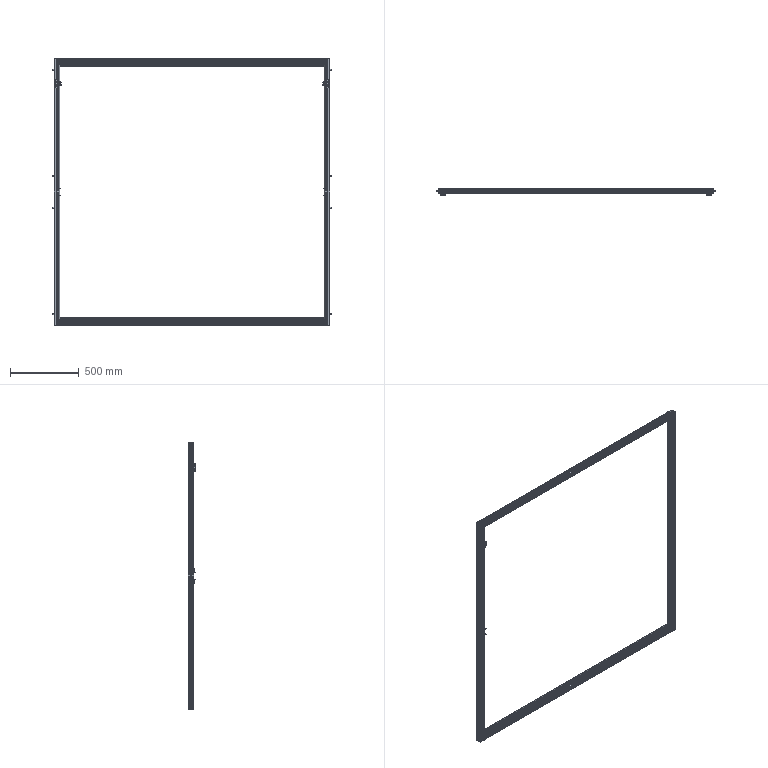Part | SolidWorks | features ReferencePattern 13, DerivedHolePattern 3, LocalLPattern 2 | 94 solids | 3410 faces | volume 5346170 mm3 | plane 2146 | cylinder 836 | cone 404 | spline 24 | commonest cylinder face diameters 6.8 x112 0.562 x80 2 x60 6 x50 10 x48 11 x48